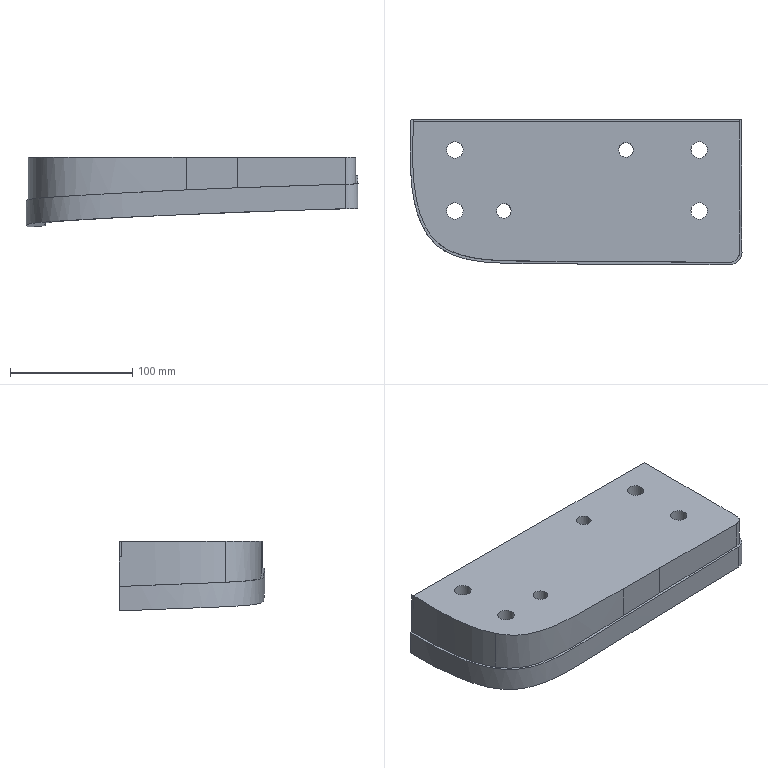Part | NX | features solid 2 | 1 solid | 34 faces | box 271.82 x 118.963 x 57.261 mm | volume 1233841 mm3 | spline 14 | plane 10 | cylinder 10 | commonest cylinder face diameters 13.5 x4 20 x4 12 x2